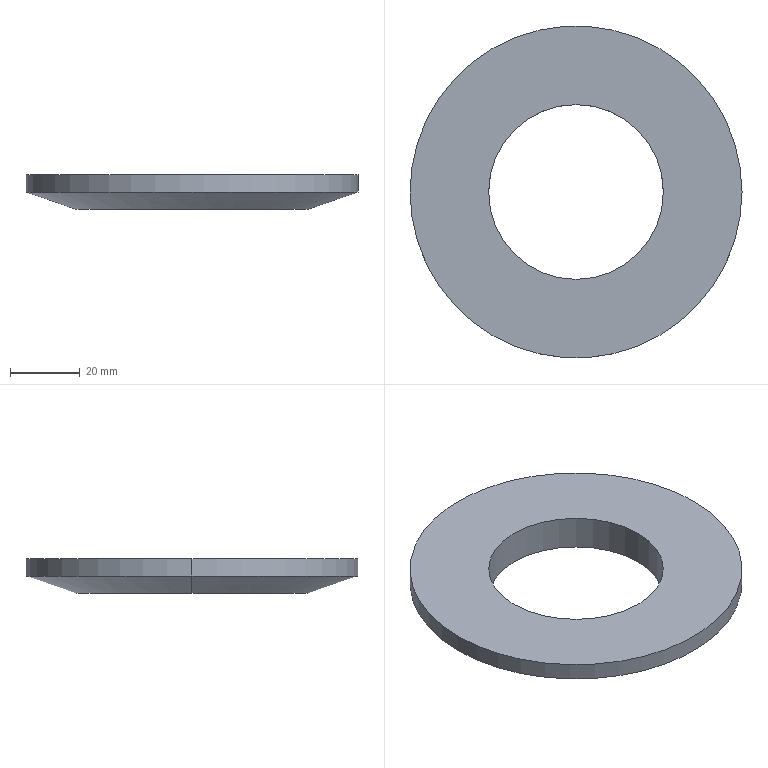Part | SolidWorks | features Revolution 1 | 1 solid | 8 faces | box 95 x 95 x 10 mm | volume 41529 mm3 | cylinder 4 | cone 2 | plane 2 | commonest cylinder face diameters 50 x2 95 x2
STEP:
#1=CARTESIAN_POINT('',(554.231,234.744,-398.998));
#2=VERTEX_POINT('',#1);
#3=CARTESIAN_POINT('',(488.231,234.744,-398.998));
#4=VERTEX_POINT('',#3);
#5=CARTESIAN_POINT('',(521.231,234.744,-398.998));
#6=DIRECTION('',(0.,0.,1.));
#7=DIRECTION('',(1.,0.,0.));
#8=AXIS2_PLACEMENT_3D('',#5,#6,#7);
#9=CIRCLE('',#8,33.);
#10=EDGE_CURVE('',#2,#4,#9,.T.);
#11=ORIENTED_EDGE('',*,*,#10,.T.);
#12=CARTESIAN_POINT('',(473.731,234.744,-393.998));
#13=VERTEX_POINT('',#12);
#14=CARTESIAN_POINT('',(473.731,234.744,-393.998));
#15=DIRECTION('',(-0.9454,0.,0.326));
#16=VECTOR('',#15,1000.);
#17=LINE('',#14,#16);
#18=EDGE_CURVE('',#4,#13,#17,.T.);
#19=ORIENTED_EDGE('',*,*,#18,.T.);
#20=CARTESIAN_POINT('',(568.731,234.744,-393.998));
#21=VERTEX_POINT('',#20);
#22=CARTESIAN_POINT('',(521.231,234.744,-393.998));
#23=DIRECTION('',(0.,0.,1.));
#24=DIRECTION('',(1.,0.,0.));
#25=AXIS2_PLACEMENT_3D('',#22,#23,#24);
#26=CIRCLE('',#25,47.5);
#27=EDGE_CURVE('',#21,#13,#26,.T.);
#28=ORIENTED_EDGE('',*,*,#27,.F.);
#29=CARTESIAN_POINT('',(568.731,234.744,-393.998));
#30=DIRECTION('',(0.9454,0.,0.326));
#31=VECTOR('',#30,1000.);
#32=LINE('',#29,#31);
#33=EDGE_CURVE('',#2,#21,#32,.T.);
#34=ORIENTED_EDGE('',*,*,#33,.F.);
#35=EDGE_LOOP('',(#11,#19,#28,#34));
#36=FACE_OUTER_BOUND('',#35,.T.);
#37=CARTESIAN_POINT('',(521.231,234.744,-393.998));
#38=DIRECTION('',(0.,0.,1.));
#39=DIRECTION('',(1.,0.,0.));
#40=AXIS2_PLACEMENT_3D('',#37,#38,#39);
#41=CONICAL_SURFACE('',#40,47.5,1.239);
#42=ADVANCED_FACE('',(#36),#41,.T.);
#43=ORIENTED_EDGE('',*,*,#27,.T.);
#44=CARTESIAN_POINT('',(473.731,234.744,-388.998));
#45=VERTEX_POINT('',#44);
#46=CARTESIAN_POINT('',(473.731,234.744,-398.998));
#47=DIRECTION('',(0.,0.,1.));
#48=VECTOR('',#47,1000.);
#49=LINE('',#46,#48);
#50=EDGE_CURVE('',#13,#45,#49,.T.);
#51=ORIENTED_EDGE('',*,*,#50,.T.);
#52=CARTESIAN_POINT('',(568.731,234.744,-388.998));
#53=VERTEX_POINT('',#52);
#54=CARTESIAN_POINT('',(521.231,234.744,-388.998));
#55=DIRECTION('',(0.,0.,1.));
#56=DIRECTION('',(1.,0.,0.));
#57=AXIS2_PLACEMENT_3D('',#54,#55,#56);
#58=CIRCLE('',#57,47.5);
#59=EDGE_CURVE('',#53,#45,#58,.T.);
#60=ORIENTED_EDGE('',*,*,#59,.F.);
#61=CARTESIAN_POINT('',(568.731,234.744,-398.998));
#62=DIRECTION('',(0.,0.,1.));
#63=VECTOR('',#62,1000.);
#64=LINE('',#61,#63);
#65=EDGE_CURVE('',#21,#53,#64,.T.);
#66=ORIENTED_EDGE('',*,*,#65,.F.);
#67=EDGE_LOOP('',(#43,#51,#60,#66));
#68=FACE_OUTER_BOUND('',#67,.T.);
#69=CARTESIAN_POINT('',(521.231,234.744,-398.998));
#70=DIRECTION('',(0.,0.,1.));
#71=DIRECTION('',(1.,0.,0.));
#72=AXIS2_PLACEMENT_3D('',#69,#70,#71);
#73=CYLINDRICAL_SURFACE('',#72,47.5);
#74=ADVANCED_FACE('',(#68),#73,.T.);
#75=CARTESIAN_POINT('',(496.231,234.744,-398.998));
#76=VERTEX_POINT('',#75);
#77=CARTESIAN_POINT('',(546.231,234.744,-398.998));
#78=VERTEX_POINT('',#77);
#79=CARTESIAN_POINT('',(521.231,234.744,-398.998));
#80=DIRECTION('',(0.,0.,1.));
#81=DIRECTION('',(1.,0.,0.));
#82=AXIS2_PLACEMENT_3D('',#79,#80,#81);
#83=CIRCLE('',#82,25.);
#84=EDGE_CURVE('',#76,#78,#83,.T.);
#85=ORIENTED_EDGE('',*,*,#84,.F.);
#86=CARTESIAN_POINT('',(496.231,234.744,-388.998));
#87=VERTEX_POINT('',#86);
#88=CARTESIAN_POINT('',(496.231,234.744,-398.998));
#89=DIRECTION('',(0.,0.,1.));
#90=VECTOR('',#89,1000.);
#91=LINE('',#88,#90);
#92=EDGE_CURVE('',#76,#87,#91,.T.);
#93=ORIENTED_EDGE('',*,*,#92,.T.);
#94=CARTESIAN_POINT('',(546.231,234.744,-388.998));
#95=VERTEX_POINT('',#94);
#96=CARTESIAN_POINT('',(521.231,234.744,-388.998));
#97=DIRECTION('',(0.,0.,1.));
#98=DIRECTION('',(1.,0.,0.));
#99=AXIS2_PLACEMENT_3D('',#96,#97,#98);
#100=CIRCLE('',#99,25.);
#101=EDGE_CURVE('',#87,#95,#100,.T.);
#102=ORIENTED_EDGE('',*,*,#101,.T.);
#103=CARTESIAN_POINT('',(546.231,234.744,-398.998));
#104=DIRECTION('',(0.,0.,1.));
#105=VECTOR('',#104,1000.);
#106=LINE('',#103,#105);
#107=EDGE_CURVE('',#78,#95,#106,.T.);
#108=ORIENTED_EDGE('',*,*,#107,.F.);
#109=EDGE_LOOP('',(#85,#93,#102,#108));
#110=FACE_OUTER_BOUND('',#109,.T.);
#111=CARTESIAN_POINT('',(521.231,234.744,-398.998));
#112=DIRECTION('',(0.,0.,1.));
#113=DIRECTION('',(1.,0.,0.));
#114=AXIS2_PLACEMENT_3D('',#111,#112,#113);
#115=CYLINDRICAL_SURFACE('',#114,25.);
#116=ADVANCED_FACE('',(#110),#115,.F.);
#117=ORIENTED_EDGE('',*,*,#92,.F.);
#118=CARTESIAN_POINT('',(521.231,234.744,-398.998));
#119=DIRECTION('',(0.,0.,1.));
#120=DIRECTION('',(1.,0.,0.));
#121=AXIS2_PLACEMENT_3D('',#118,#119,#120);
#122=CIRCLE('',#121,25.);
#123=EDGE_CURVE('',#78,#76,#122,.T.);
#124=ORIENTED_EDGE('',*,*,#123,.F.);
#125=ORIENTED_EDGE('',*,*,#107,.T.);
#126=CARTESIAN_POINT('',(521.231,234.744,-388.998));
#127=DIRECTION('',(0.,0.,1.));
#128=DIRECTION('',(1.,0.,0.));
#129=AXIS2_PLACEMENT_3D('',#126,#127,#128);
#130=CIRCLE('',#129,25.);
#131=EDGE_CURVE('',#95,#87,#130,.T.);
#132=ORIENTED_EDGE('',*,*,#131,.T.);
#133=EDGE_LOOP('',(#117,#124,#125,#132));
#134=FACE_OUTER_BOUND('',#133,.T.);
#135=CARTESIAN_POINT('',(521.231,234.744,-398.998));
#136=DIRECTION('',(0.,0.,1.));
#137=DIRECTION('',(1.,0.,0.));
#138=AXIS2_PLACEMENT_3D('',#135,#136,#137);
#139=CYLINDRICAL_SURFACE('',#138,25.);
#140=ADVANCED_FACE('',(#134),#139,.F.);
#141=ORIENTED_EDGE('',*,*,#59,.T.);
#142=CARTESIAN_POINT('',(521.231,234.744,-388.998));
#143=DIRECTION('',(0.,0.,1.));
#144=DIRECTION('',(1.,0.,0.));
#145=AXIS2_PLACEMENT_3D('',#142,#143,#144);
#146=CIRCLE('',#145,47.5);
#147=EDGE_CURVE('',#45,#53,#146,.T.);
#148=ORIENTED_EDGE('',*,*,#147,.T.);
#149=EDGE_LOOP('',(#141,#148));
#150=FACE_OUTER_BOUND('',#149,.T.);
#151=ORIENTED_EDGE('',*,*,#131,.F.);
#152=ORIENTED_EDGE('',*,*,#101,.F.);
#153=EDGE_LOOP('',(#151,#152));
#154=FACE_BOUND('',#153,.T.);
#155=CARTESIAN_POINT('',(546.231,234.744,-388.998));
#156=DIRECTION('',(0.,0.,1.));
#157=DIRECTION('',(1.,0.,0.));
#158=AXIS2_PLACEMENT_3D('',#155,#156,#157);
#159=PLANE('',#158);
#160=ADVANCED_FACE('',(#150,#154),#159,.T.);
#161=ORIENTED_EDGE('',*,*,#50,.F.);
#162=CARTESIAN_POINT('',(521.231,234.744,-393.998));
#163=DIRECTION('',(0.,0.,1.));
#164=DIRECTION('',(1.,0.,0.));
#165=AXIS2_PLACEMENT_3D('',#162,#163,#164);
#166=CIRCLE('',#165,47.5);
#167=EDGE_CURVE('',#13,#21,#166,.T.);
#168=ORIENTED_EDGE('',*,*,#167,.T.);
#169=ORIENTED_EDGE('',*,*,#65,.T.);
#170=ORIENTED_EDGE('',*,*,#147,.F.);
#171=EDGE_LOOP('',(#161,#168,#169,#170));
#172=FACE_OUTER_BOUND('',#171,.T.);
#173=CARTESIAN_POINT('',(521.231,234.744,-398.998));
#174=DIRECTION('',(0.,0.,1.));
#175=DIRECTION('',(1.,0.,0.));
#176=AXIS2_PLACEMENT_3D('',#173,#174,#175);
#177=CYLINDRICAL_SURFACE('',#176,47.5);
#178=ADVANCED_FACE('',(#172),#177,.T.);
#179=ORIENTED_EDGE('',*,*,#18,.F.);
#180=CARTESIAN_POINT('',(521.231,234.744,-398.998));
#181=DIRECTION('',(0.,0.,1.));
#182=DIRECTION('',(1.,0.,0.));
#183=AXIS2_PLACEMENT_3D('',#180,#181,#182);
#184=CIRCLE('',#183,33.);
#185=EDGE_CURVE('',#4,#2,#184,.T.);
#186=ORIENTED_EDGE('',*,*,#185,.T.);
#187=ORIENTED_EDGE('',*,*,#33,.T.);
#188=ORIENTED_EDGE('',*,*,#167,.F.);
#189=EDGE_LOOP('',(#179,#186,#187,#188));
#190=FACE_OUTER_BOUND('',#189,.T.);
#191=CARTESIAN_POINT('',(521.231,234.744,-393.998));
#192=DIRECTION('',(0.,0.,1.));
#193=DIRECTION('',(1.,0.,0.));
#194=AXIS2_PLACEMENT_3D('',#191,#192,#193);
#195=CONICAL_SURFACE('',#194,47.5,1.239);
#196=ADVANCED_FACE('',(#190),#195,.T.);
#197=ORIENTED_EDGE('',*,*,#123,.T.);
#198=ORIENTED_EDGE('',*,*,#84,.T.);
#199=EDGE_LOOP('',(#197,#198));
#200=FACE_BOUND('',#199,.T.);
#201=ORIENTED_EDGE('',*,*,#10,.F.);
#202=ORIENTED_EDGE('',*,*,#185,.F.);
#203=EDGE_LOOP('',(#201,#202));
#204=FACE_OUTER_BOUND('',#203,.T.);
#205=CARTESIAN_POINT('',(554.231,234.744,-398.998));
#206=DIRECTION('',(0.,0.,-1.));
#207=DIRECTION('',(-1.,0.,0.));
#208=AXIS2_PLACEMENT_3D('',#205,#206,#207);
#209=PLANE('',#208);
#210=ADVANCED_FACE('',(#200,#204),#209,.T.);
#211=CLOSED_SHELL('',(#42,#74,#116,#140,#160,#178,#196,#210));
#212=MANIFOLD_SOLID_BREP('',#211);
#213=CARTESIAN_POINT('',(0.,0.,0.));
#214=DIRECTION('',(0.,0.,1.));
#215=DIRECTION('',(1.,0.,0.));
#216=AXIS2_PLACEMENT_3D('',#213,#214,#215);
#217=(LENGTH_UNIT()NAMED_UNIT(*)SI_UNIT(.MILLI.,.METRE.));
#218=UNCERTAINTY_MEASURE_WITH_UNIT(LENGTH_MEASURE(0.00001),#217,'','');
#219=(NAMED_UNIT(*)PLANE_ANGLE_UNIT()SI_UNIT($,.RADIAN.));
#220=(NAMED_UNIT(*)SI_UNIT($,.STERADIAN.)SOLID_ANGLE_UNIT());
#221=(GEOMETRIC_REPRESENTATION_CONTEXT(3)GLOBAL_UNCERTAINTY_ASSIGNED_CONTEXT((#218))GLOBAL_UNIT_ASSIGNED_CONTEXT((#217,#219,#220))REPRESENTATION_CONTEXT('',''));
#222=ADVANCED_BREP_SHAPE_REPRESENTATION('',(#212,#216),#221);